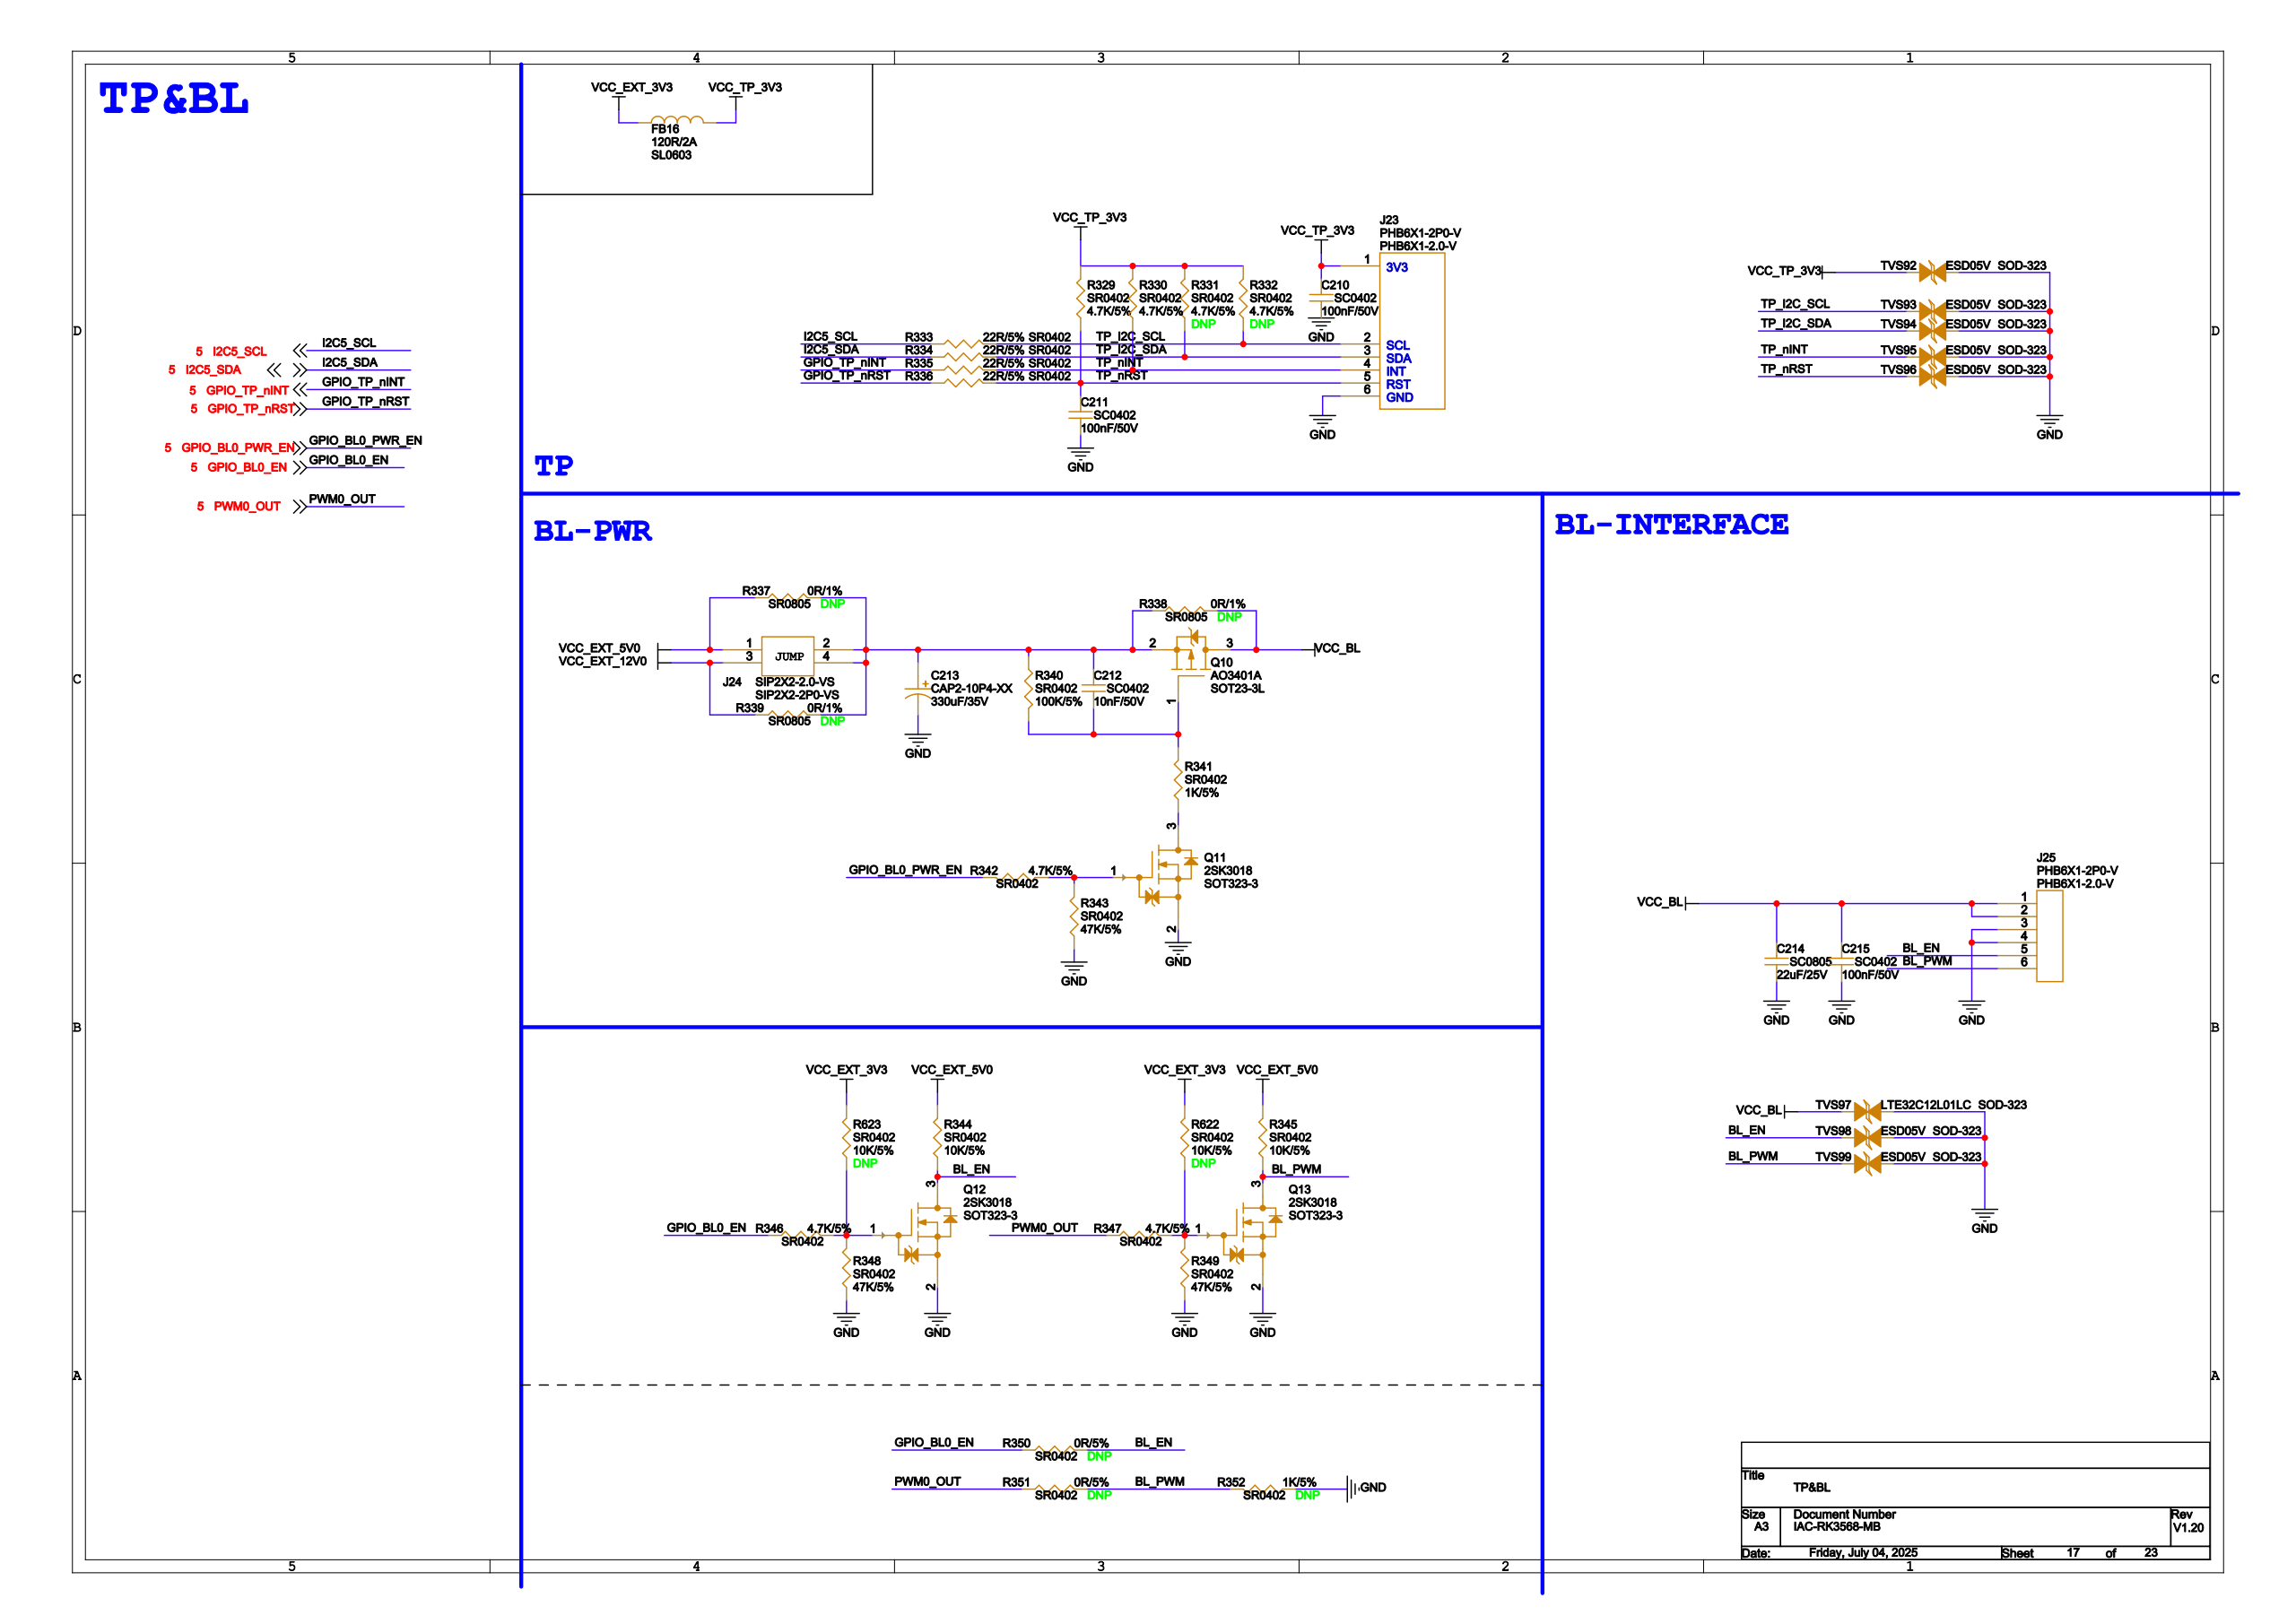Circuit board | Cadence Allegro | 1138 parts | 722 nets | one sheet of the schematic
Parts on this sheet (reference | value | footprint):
C210 | 100nF/50V | SC0402
C211 | 100nF/50V | SC0402
C212 | 10nF/50V | SC0402
C213 | 330uF/35V | CAP2-10P4-XX
C214 | 22uF/25V | SC0805
C215 | 100nF/50V | SC0402
FB16 | 120R/2A | SL0603
J23 | PHB6X1-2.0-V | PHB6X1-2P0-V
J24 | SIP2X2-2.0-VS | SIP2X2-2P0-VS
J25 | PHB6X1-2.0-V | PHB6X1-2P0-V
Q10 | AO3401A | SOT23-3L
Q11 | 2SK3018 | SOT323-3
Q12 | 2SK3018 | SOT323-3
Q13 | 2SK3018 | SOT323-3
R329 | 4.7K/5% | SR0402
R330 | 4.7K/5% | SR0402
R331 | 4.7K/5% | SR0402
R332 | 4.7K/5% | SR0402
R333 | 22R/5% | SR0402
R334 | 22R/5% | SR0402
R335 | 22R/5% | SR0402
R336 | 22R/5% | SR0402
R337 | 0R/1% | SR0805
R338 | 0R/1% | SR0805
R339 | 0R/1% | SR0805
R340 | 100K/5% | SR0402
R341 | 1K/5% | SR0402
R342 | 4.7K/5% | SR0402
R343 | 47K/5% | SR0402
R344 | 10K/5% | SR0402
R345 | 10K/5% | SR0402
R346 | 4.7K/5% | SR0402
R347 | 4.7K/5% | SR0402
R348 | 47K/5% | SR0402
R349 | 47K/5% | SR0402
R350 | 0R/5% | SR0402
R351 | 0R/5% | SR0402
R352 | 1K/5% | SR0402
R622 | 10K/5% | SR0402
R623 | 10K/5% | SR0402
TVS92 | ESD05V | SOD-323
TVS93 | ESD05V | SOD-323
TVS94 | ESD05V | SOD-323
TVS95 | ESD05V | SOD-323
TVS96 | ESD05V | SOD-323
TVS97 | LTE32C12L01LC | SOD-323
TVS98 | ESD05V | SOD-323
TVS99 | ESD05V | SOD-323
Nets of these parts (net: part-pin ...):
VCC_EXT_5V0: J24-1 R337-1 R344-2 R345-2
VCC_EXT_3V3: FB16-1 R622-2 R623-2
GND: C210-2 C211-2 C213-2 C214-2 C215-2 J23-6 J25-3 J25-4 Q11-2 Q12-2 Q13-2 R343-1 R348-1 R349-1 R352-1 TVS92-2 TVS93-2 TVS94-2 TVS95-2 TVS96-2 TVS97-2 TVS98-2 TVS99-2
VCC_TP_3V3: C210-1 FB16-2 J23-1 R329-2 R330-2 R331-2 R332-2 TVS92-1
TP_I2C_SCL: J23-2 R332-1 R333-2 TVS93-1
TP_I2C_SDA: J23-3 R331-1 R334-2 TVS94-1
TP_NINT: J23-4 R330-1 R335-2 TVS95-1
TP_NRST: C211-1 J23-5 R329-1 R336-2 TVS96-1
BL_EN: J25-5 Q12-3 R344-1 R350-2 TVS98-1
BL_PWM: J25-6 Q13-3 R345-1 R351-2 R352-2 TVS99-1
VCC_BL: C214-1 C215-1 J25-1 J25-2 Q10-3 R338-2 TVS97-1
N7217533: C212-2 Q10-1 R340-2 R341-2
N4547766: C212-1 C213-1 J24-2 J24-4 Q10-2 R337-2 R338-1 R339-2 R340-1
N19587072: Q11-3 R341-1
N19587121: Q11-1 R342-1 R343-2
N6351752: Q12-1 R346-2 R348-2 R623-1
N6351696: Q13-1 R347-2 R349-2 R622-1
VCC_EXT_12V0: J24-3 R339-1
PWM0_OUT: R347-1 R351-1
I2C5_SCL: R333-1
I2C5_SDA: R334-1
GPIO_TP_NRST: R336-1
GPIO_TP_NINT: R335-1
GPIO_BL0_PWR_EN: R342-2
GPIO_BL0_EN: R346-1 R350-1